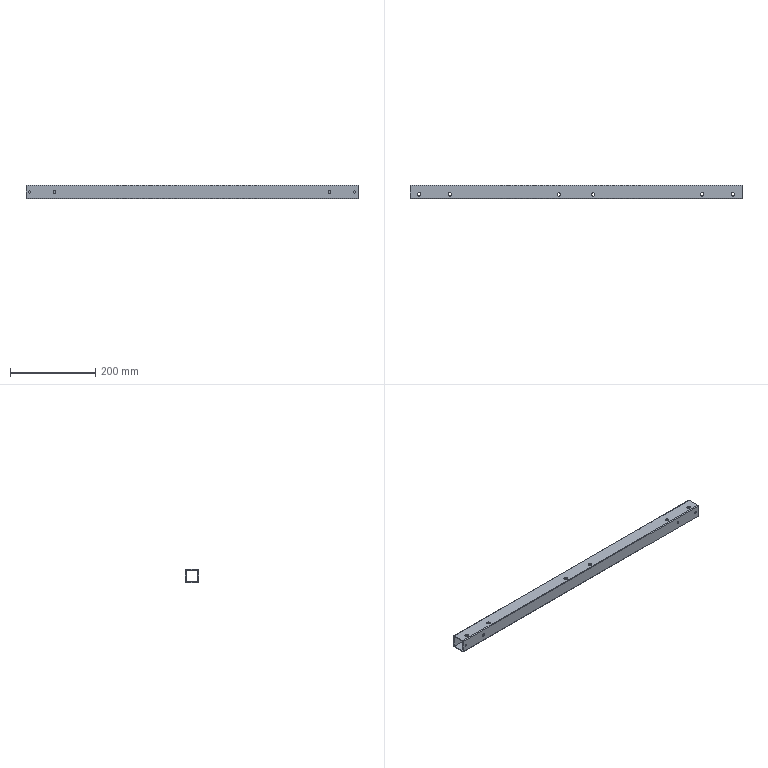Part | NX | features BREP 1 | 1 solid | 46 faces | box 780.288 x 31.75 x 31.75 mm | volume 172182 mm3 | cylinder 36 | plane 10 | commonest cylinder face diameters 8.128 x24 3.175 x4 5.08 x4 6.35 x4